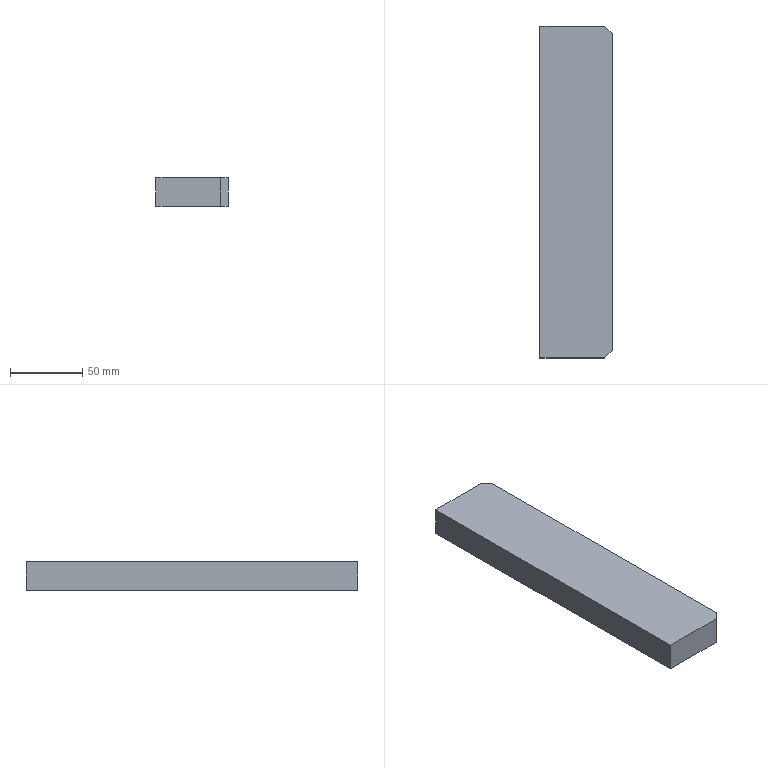Part | STEP file | Tube necking machine_id722_x_t | 1 solid | 8 faces | box 50 x 230 x 20 mm | volume 229500 mm3 | plane 8
STEP:
#1=CARTESIAN_POINT('',(0.,0.,0.));
#2=DIRECTION('',(0.,0.,1.));
#3=DIRECTION('',(1.,0.,0.));
#4=AXIS2_PLACEMENT_3D('',#1,#2,#3);
#5=CARTESIAN_POINT('',(222.5,-271.,20.));
#6=VERTEX_POINT('',#5);
#7=CARTESIAN_POINT('',(222.5,-51.,20.));
#8=VERTEX_POINT('',#7);
#9=CARTESIAN_POINT('',(222.5,-46.,20.));
#10=DIRECTION('',(0.,1.,0.));
#11=VECTOR('',#10,1.);
#12=LINE('',#9,#11);
#13=CARTESIAN_POINT('',(222.5,-46.,20.));
#14=DIRECTION('',(-1.,0.,0.));
#15=DIRECTION('',(0.,1.,0.));
#16=AXIS2_PLACEMENT_3D('',#13,#14,#15);
#17=PLANE('',#16);
#18=CARTESIAN_POINT('',(0.,0.));
#19=DIRECTION('',(1.,0.));
#20=VECTOR('',#19,1.);
#21=LINE('',#18,#20);
#22=(GEOMETRIC_REPRESENTATION_CONTEXT(2)PARAMETRIC_REPRESENTATION_CONTEXT()REPRESENTATION_CONTEXT('',''));
#23=DEFINITIONAL_REPRESENTATION('',(#21),#22);
#24=PCURVE('',#17,#23);
#25=CARTESIAN_POINT('',(0.,0.,20.));
#26=DIRECTION('',(0.,0.,1.));
#27=DIRECTION('',(-1.,0.,0.));
#28=AXIS2_PLACEMENT_3D('',#25,#26,#27);
#29=PLANE('',#28);
#30=CARTESIAN_POINT('',(-222.5,46.));
#31=DIRECTION('',(0.,-1.));
#32=VECTOR('',#31,1.);
#33=LINE('',#30,#32);
#34=(GEOMETRIC_REPRESENTATION_CONTEXT(2)PARAMETRIC_REPRESENTATION_CONTEXT()REPRESENTATION_CONTEXT('',''));
#35=DEFINITIONAL_REPRESENTATION('',(#33),#34);
#36=PCURVE('',#29,#35);
#37=SURFACE_CURVE('',#12,(#24,#36),.PCURVE_S1.);
#38=EDGE_CURVE('',#6,#8,#37,.T.);
#39=ORIENTED_EDGE('',*,*,#38,.F.);
#40=CARTESIAN_POINT('',(222.5,-271.,0.));
#41=VERTEX_POINT('',#40);
#42=CARTESIAN_POINT('',(222.5,-271.,20.));
#43=DIRECTION('',(0.,0.,-1.));
#44=VECTOR('',#43,1.);
#45=LINE('',#42,#44);
#46=CARTESIAN_POINT('',(-225.,0.));
#47=DIRECTION('',(0.,1.));
#48=VECTOR('',#47,1.);
#49=LINE('',#46,#48);
#50=(GEOMETRIC_REPRESENTATION_CONTEXT(2)PARAMETRIC_REPRESENTATION_CONTEXT()REPRESENTATION_CONTEXT('',''));
#51=DEFINITIONAL_REPRESENTATION('',(#49),#50);
#52=PCURVE('',#17,#51);
#53=CARTESIAN_POINT('',(217.5,-276.,20.));
#54=DIRECTION('',(-0.7071,0.7071,0.));
#55=DIRECTION('',(0.,0.,-1.));
#56=AXIS2_PLACEMENT_3D('',#53,#54,#55);
#57=PLANE('',#56);
#58=CARTESIAN_POINT('',(0.,-7.071));
#59=DIRECTION('',(1.,0.));
#60=VECTOR('',#59,1.);
#61=LINE('',#58,#60);
#62=(GEOMETRIC_REPRESENTATION_CONTEXT(2)PARAMETRIC_REPRESENTATION_CONTEXT()REPRESENTATION_CONTEXT('',''));
#63=DEFINITIONAL_REPRESENTATION('',(#61),#62);
#64=PCURVE('',#57,#63);
#65=SURFACE_CURVE('',#45,(#52,#64),.PCURVE_S1.);
#66=EDGE_CURVE('',#6,#41,#65,.T.);
#67=ORIENTED_EDGE('',*,*,#66,.T.);
#68=CARTESIAN_POINT('',(222.5,-51.,0.));
#69=VERTEX_POINT('',#68);
#70=CARTESIAN_POINT('',(222.5,-46.,0.));
#71=DIRECTION('',(0.,1.,0.));
#72=VECTOR('',#71,1.);
#73=LINE('',#70,#72);
#74=CARTESIAN_POINT('',(0.,20.));
#75=DIRECTION('',(1.,0.));
#76=VECTOR('',#75,1.);
#77=LINE('',#74,#76);
#78=(GEOMETRIC_REPRESENTATION_CONTEXT(2)PARAMETRIC_REPRESENTATION_CONTEXT()REPRESENTATION_CONTEXT('',''));
#79=DEFINITIONAL_REPRESENTATION('',(#77),#78);
#80=PCURVE('',#17,#79);
#81=CARTESIAN_POINT('',(0.,0.,0.));
#82=DIRECTION('',(0.,0.,1.));
#83=DIRECTION('',(-1.,0.,0.));
#84=AXIS2_PLACEMENT_3D('',#81,#82,#83);
#85=PLANE('',#84);
#86=CARTESIAN_POINT('',(-222.5,46.));
#87=DIRECTION('',(0.,-1.));
#88=VECTOR('',#87,1.);
#89=LINE('',#86,#88);
#90=(GEOMETRIC_REPRESENTATION_CONTEXT(2)PARAMETRIC_REPRESENTATION_CONTEXT()REPRESENTATION_CONTEXT('',''));
#91=DEFINITIONAL_REPRESENTATION('',(#89),#90);
#92=PCURVE('',#85,#91);
#93=SURFACE_CURVE('',#73,(#80,#92),.PCURVE_S1.);
#94=EDGE_CURVE('',#41,#69,#93,.T.);
#95=ORIENTED_EDGE('',*,*,#94,.T.);
#96=CARTESIAN_POINT('',(222.5,-51.,20.));
#97=DIRECTION('',(0.,0.,1.));
#98=VECTOR('',#97,1.);
#99=LINE('',#96,#98);
#100=CARTESIAN_POINT('',(-5.,0.));
#101=DIRECTION('',(0.,-1.));
#102=VECTOR('',#101,1.);
#103=LINE('',#100,#102);
#104=(GEOMETRIC_REPRESENTATION_CONTEXT(2)PARAMETRIC_REPRESENTATION_CONTEXT()REPRESENTATION_CONTEXT('',''));
#105=DEFINITIONAL_REPRESENTATION('',(#103),#104);
#106=PCURVE('',#17,#105);
#107=CARTESIAN_POINT('',(222.5,-51.,20.));
#108=DIRECTION('',(-0.7071,-0.7071,0.));
#109=DIRECTION('',(0.,0.,-1.));
#110=AXIS2_PLACEMENT_3D('',#107,#108,#109);
#111=PLANE('',#110);
#112=CARTESIAN_POINT('',(0.,0.));
#113=DIRECTION('',(-1.,0.));
#114=VECTOR('',#113,1.);
#115=LINE('',#112,#114);
#116=(GEOMETRIC_REPRESENTATION_CONTEXT(2)PARAMETRIC_REPRESENTATION_CONTEXT()REPRESENTATION_CONTEXT('',''));
#117=DEFINITIONAL_REPRESENTATION('',(#115),#116);
#118=PCURVE('',#111,#117);
#119=SURFACE_CURVE('',#99,(#106,#118),.PCURVE_S1.);
#120=EDGE_CURVE('',#69,#8,#119,.T.);
#121=ORIENTED_EDGE('',*,*,#120,.T.);
#122=EDGE_LOOP('',(#39,#67,#95,#121));
#123=FACE_BOUND('',#122,.T.);
#124=ADVANCED_FACE('',(#123),#17,.F.);
#125=CARTESIAN_POINT('',(172.5,-276.,20.));
#126=VERTEX_POINT('',#125);
#127=CARTESIAN_POINT('',(217.5,-276.,20.));
#128=VERTEX_POINT('',#127);
#129=CARTESIAN_POINT('',(222.5,-276.,20.));
#130=DIRECTION('',(1.,0.,0.));
#131=VECTOR('',#130,1.);
#132=LINE('',#129,#131);
#133=CARTESIAN_POINT('',(222.5,-276.,20.));
#134=DIRECTION('',(0.,1.,0.));
#135=DIRECTION('',(1.,0.,0.));
#136=AXIS2_PLACEMENT_3D('',#133,#134,#135);
#137=PLANE('',#136);
#138=CARTESIAN_POINT('',(0.,0.));
#139=DIRECTION('',(1.,0.));
#140=VECTOR('',#139,1.);
#141=LINE('',#138,#140);
#142=(GEOMETRIC_REPRESENTATION_CONTEXT(2)PARAMETRIC_REPRESENTATION_CONTEXT()REPRESENTATION_CONTEXT('',''));
#143=DEFINITIONAL_REPRESENTATION('',(#141),#142);
#144=PCURVE('',#137,#143);
#145=CARTESIAN_POINT('',(-222.5,276.));
#146=DIRECTION('',(-1.,0.));
#147=VECTOR('',#146,1.);
#148=LINE('',#145,#147);
#149=(GEOMETRIC_REPRESENTATION_CONTEXT(2)PARAMETRIC_REPRESENTATION_CONTEXT()REPRESENTATION_CONTEXT('',''));
#150=DEFINITIONAL_REPRESENTATION('',(#148),#149);
#151=PCURVE('',#29,#150);
#152=SURFACE_CURVE('',#132,(#144,#151),.PCURVE_S1.);
#153=EDGE_CURVE('',#126,#128,#152,.T.);
#154=ORIENTED_EDGE('',*,*,#153,.F.);
#155=CARTESIAN_POINT('',(172.5,-276.,0.));
#156=VERTEX_POINT('',#155);
#157=CARTESIAN_POINT('',(172.5,-276.,20.));
#158=DIRECTION('',(0.,0.,1.));
#159=VECTOR('',#158,1.);
#160=LINE('',#157,#159);
#161=CARTESIAN_POINT('',(-50.,0.));
#162=DIRECTION('',(0.,-1.));
#163=VECTOR('',#162,1.);
#164=LINE('',#161,#163);
#165=(GEOMETRIC_REPRESENTATION_CONTEXT(2)PARAMETRIC_REPRESENTATION_CONTEXT()REPRESENTATION_CONTEXT('',''));
#166=DEFINITIONAL_REPRESENTATION('',(#164),#165);
#167=PCURVE('',#137,#166);
#168=CARTESIAN_POINT('',(172.5,-276.,20.));
#169=DIRECTION('',(1.,0.,0.));
#170=DIRECTION('',(0.,-1.,0.));
#171=AXIS2_PLACEMENT_3D('',#168,#169,#170);
#172=PLANE('',#171);
#173=CARTESIAN_POINT('',(0.,0.));
#174=DIRECTION('',(0.,-1.));
#175=VECTOR('',#174,1.);
#176=LINE('',#173,#175);
#177=(GEOMETRIC_REPRESENTATION_CONTEXT(2)PARAMETRIC_REPRESENTATION_CONTEXT()REPRESENTATION_CONTEXT('',''));
#178=DEFINITIONAL_REPRESENTATION('',(#176),#177);
#179=PCURVE('',#172,#178);
#180=SURFACE_CURVE('',#160,(#167,#179),.PCURVE_S1.);
#181=EDGE_CURVE('',#156,#126,#180,.T.);
#182=ORIENTED_EDGE('',*,*,#181,.F.);
#183=CARTESIAN_POINT('',(217.5,-276.,0.));
#184=VERTEX_POINT('',#183);
#185=CARTESIAN_POINT('',(222.5,-276.,0.));
#186=DIRECTION('',(1.,0.,0.));
#187=VECTOR('',#186,1.);
#188=LINE('',#185,#187);
#189=CARTESIAN_POINT('',(0.,20.));
#190=DIRECTION('',(1.,0.));
#191=VECTOR('',#190,1.);
#192=LINE('',#189,#191);
#193=(GEOMETRIC_REPRESENTATION_CONTEXT(2)PARAMETRIC_REPRESENTATION_CONTEXT()REPRESENTATION_CONTEXT('',''));
#194=DEFINITIONAL_REPRESENTATION('',(#192),#193);
#195=PCURVE('',#137,#194);
#196=CARTESIAN_POINT('',(-222.5,276.));
#197=DIRECTION('',(-1.,0.));
#198=VECTOR('',#197,1.);
#199=LINE('',#196,#198);
#200=(GEOMETRIC_REPRESENTATION_CONTEXT(2)PARAMETRIC_REPRESENTATION_CONTEXT()REPRESENTATION_CONTEXT('',''));
#201=DEFINITIONAL_REPRESENTATION('',(#199),#200);
#202=PCURVE('',#85,#201);
#203=SURFACE_CURVE('',#188,(#195,#202),.PCURVE_S1.);
#204=EDGE_CURVE('',#156,#184,#203,.T.);
#205=ORIENTED_EDGE('',*,*,#204,.T.);
#206=CARTESIAN_POINT('',(217.5,-276.,20.));
#207=DIRECTION('',(0.,0.,1.));
#208=VECTOR('',#207,1.);
#209=LINE('',#206,#208);
#210=CARTESIAN_POINT('',(-5.,0.));
#211=DIRECTION('',(0.,-1.));
#212=VECTOR('',#211,1.);
#213=LINE('',#210,#212);
#214=(GEOMETRIC_REPRESENTATION_CONTEXT(2)PARAMETRIC_REPRESENTATION_CONTEXT()REPRESENTATION_CONTEXT('',''));
#215=DEFINITIONAL_REPRESENTATION('',(#213),#214);
#216=PCURVE('',#137,#215);
#217=CARTESIAN_POINT('',(0.,0.));
#218=DIRECTION('',(-1.,0.));
#219=VECTOR('',#218,1.);
#220=LINE('',#217,#219);
#221=(GEOMETRIC_REPRESENTATION_CONTEXT(2)PARAMETRIC_REPRESENTATION_CONTEXT()REPRESENTATION_CONTEXT('',''));
#222=DEFINITIONAL_REPRESENTATION('',(#220),#221);
#223=PCURVE('',#57,#222);
#224=SURFACE_CURVE('',#209,(#216,#223),.PCURVE_S1.);
#225=EDGE_CURVE('',#184,#128,#224,.T.);
#226=ORIENTED_EDGE('',*,*,#225,.T.);
#227=EDGE_LOOP('',(#154,#182,#205,#226));
#228=FACE_BOUND('',#227,.T.);
#229=ADVANCED_FACE('',(#228),#137,.F.);
#230=CARTESIAN_POINT('',(172.5,-46.,0.));
#231=VERTEX_POINT('',#230);
#232=CARTESIAN_POINT('',(172.5,-276.,0.));
#233=DIRECTION('',(0.,-1.,0.));
#234=VECTOR('',#233,1.);
#235=LINE('',#232,#234);
#236=CARTESIAN_POINT('',(0.,20.));
#237=DIRECTION('',(1.,0.));
#238=VECTOR('',#237,1.);
#239=LINE('',#236,#238);
#240=(GEOMETRIC_REPRESENTATION_CONTEXT(2)PARAMETRIC_REPRESENTATION_CONTEXT()REPRESENTATION_CONTEXT('',''));
#241=DEFINITIONAL_REPRESENTATION('',(#239),#240);
#242=PCURVE('',#172,#241);
#243=CARTESIAN_POINT('',(-172.5,276.));
#244=DIRECTION('',(0.,1.));
#245=VECTOR('',#244,1.);
#246=LINE('',#243,#245);
#247=(GEOMETRIC_REPRESENTATION_CONTEXT(2)PARAMETRIC_REPRESENTATION_CONTEXT()REPRESENTATION_CONTEXT('',''));
#248=DEFINITIONAL_REPRESENTATION('',(#246),#247);
#249=PCURVE('',#85,#248);
#250=SURFACE_CURVE('',#235,(#242,#249),.PCURVE_S1.);
#251=EDGE_CURVE('',#231,#156,#250,.T.);
#252=ORIENTED_EDGE('',*,*,#251,.T.);
#253=ORIENTED_EDGE('',*,*,#181,.T.);
#254=CARTESIAN_POINT('',(172.5,-46.,20.));
#255=VERTEX_POINT('',#254);
#256=CARTESIAN_POINT('',(172.5,-276.,20.));
#257=DIRECTION('',(0.,-1.,0.));
#258=VECTOR('',#257,1.);
#259=LINE('',#256,#258);
#260=CARTESIAN_POINT('',(0.,0.));
#261=DIRECTION('',(1.,0.));
#262=VECTOR('',#261,1.);
#263=LINE('',#260,#262);
#264=(GEOMETRIC_REPRESENTATION_CONTEXT(2)PARAMETRIC_REPRESENTATION_CONTEXT()REPRESENTATION_CONTEXT('',''));
#265=DEFINITIONAL_REPRESENTATION('',(#263),#264);
#266=PCURVE('',#172,#265);
#267=CARTESIAN_POINT('',(-172.5,276.));
#268=DIRECTION('',(0.,1.));
#269=VECTOR('',#268,1.);
#270=LINE('',#267,#269);
#271=(GEOMETRIC_REPRESENTATION_CONTEXT(2)PARAMETRIC_REPRESENTATION_CONTEXT()REPRESENTATION_CONTEXT('',''));
#272=DEFINITIONAL_REPRESENTATION('',(#270),#271);
#273=PCURVE('',#29,#272);
#274=SURFACE_CURVE('',#259,(#266,#273),.PCURVE_S1.);
#275=EDGE_CURVE('',#255,#126,#274,.T.);
#276=ORIENTED_EDGE('',*,*,#275,.F.);
#277=CARTESIAN_POINT('',(172.5,-46.,20.));
#278=DIRECTION('',(0.,0.,1.));
#279=VECTOR('',#278,1.);
#280=LINE('',#277,#279);
#281=CARTESIAN_POINT('',(-230.,0.));
#282=DIRECTION('',(0.,-1.));
#283=VECTOR('',#282,1.);
#284=LINE('',#281,#283);
#285=(GEOMETRIC_REPRESENTATION_CONTEXT(2)PARAMETRIC_REPRESENTATION_CONTEXT()REPRESENTATION_CONTEXT('',''));
#286=DEFINITIONAL_REPRESENTATION('',(#284),#285);
#287=PCURVE('',#172,#286);
#288=CARTESIAN_POINT('',(172.5,-46.,20.));
#289=DIRECTION('',(0.,-1.,0.));
#290=DIRECTION('',(-1.,0.,0.));
#291=AXIS2_PLACEMENT_3D('',#288,#289,#290);
#292=PLANE('',#291);
#293=CARTESIAN_POINT('',(0.,0.));
#294=DIRECTION('',(0.,-1.));
#295=VECTOR('',#294,1.);
#296=LINE('',#293,#295);
#297=(GEOMETRIC_REPRESENTATION_CONTEXT(2)PARAMETRIC_REPRESENTATION_CONTEXT()REPRESENTATION_CONTEXT('',''));
#298=DEFINITIONAL_REPRESENTATION('',(#296),#297);
#299=PCURVE('',#292,#298);
#300=SURFACE_CURVE('',#280,(#287,#299),.PCURVE_S1.);
#301=EDGE_CURVE('',#231,#255,#300,.T.);
#302=ORIENTED_EDGE('',*,*,#301,.F.);
#303=EDGE_LOOP('',(#252,#253,#276,#302));
#304=FACE_BOUND('',#303,.T.);
#305=ADVANCED_FACE('',(#304),#172,.F.);
#306=CARTESIAN_POINT('',(217.5,-46.,0.));
#307=VERTEX_POINT('',#306);
#308=CARTESIAN_POINT('',(172.5,-46.,0.));
#309=DIRECTION('',(-1.,0.,0.));
#310=VECTOR('',#309,1.);
#311=LINE('',#308,#310);
#312=CARTESIAN_POINT('',(0.,20.));
#313=DIRECTION('',(1.,0.));
#314=VECTOR('',#313,1.);
#315=LINE('',#312,#314);
#316=(GEOMETRIC_REPRESENTATION_CONTEXT(2)PARAMETRIC_REPRESENTATION_CONTEXT()REPRESENTATION_CONTEXT('',''));
#317=DEFINITIONAL_REPRESENTATION('',(#315),#316);
#318=PCURVE('',#292,#317);
#319=CARTESIAN_POINT('',(-172.5,46.));
#320=DIRECTION('',(1.,0.));
#321=VECTOR('',#320,1.);
#322=LINE('',#319,#321);
#323=(GEOMETRIC_REPRESENTATION_CONTEXT(2)PARAMETRIC_REPRESENTATION_CONTEXT()REPRESENTATION_CONTEXT('',''));
#324=DEFINITIONAL_REPRESENTATION('',(#322),#323);
#325=PCURVE('',#85,#324);
#326=SURFACE_CURVE('',#311,(#318,#325),.PCURVE_S1.);
#327=EDGE_CURVE('',#307,#231,#326,.T.);
#328=ORIENTED_EDGE('',*,*,#327,.T.);
#329=ORIENTED_EDGE('',*,*,#301,.T.);
#330=CARTESIAN_POINT('',(217.5,-46.,20.));
#331=VERTEX_POINT('',#330);
#332=CARTESIAN_POINT('',(172.5,-46.,20.));
#333=DIRECTION('',(-1.,0.,0.));
#334=VECTOR('',#333,1.);
#335=LINE('',#332,#334);
#336=CARTESIAN_POINT('',(0.,0.));
#337=DIRECTION('',(1.,0.));
#338=VECTOR('',#337,1.);
#339=LINE('',#336,#338);
#340=(GEOMETRIC_REPRESENTATION_CONTEXT(2)PARAMETRIC_REPRESENTATION_CONTEXT()REPRESENTATION_CONTEXT('',''));
#341=DEFINITIONAL_REPRESENTATION('',(#339),#340);
#342=PCURVE('',#292,#341);
#343=CARTESIAN_POINT('',(-172.5,46.));
#344=DIRECTION('',(1.,0.));
#345=VECTOR('',#344,1.);
#346=LINE('',#343,#345);
#347=(GEOMETRIC_REPRESENTATION_CONTEXT(2)PARAMETRIC_REPRESENTATION_CONTEXT()REPRESENTATION_CONTEXT('',''));
#348=DEFINITIONAL_REPRESENTATION('',(#346),#347);
#349=PCURVE('',#29,#348);
#350=SURFACE_CURVE('',#335,(#342,#349),.PCURVE_S1.);
#351=EDGE_CURVE('',#331,#255,#350,.T.);
#352=ORIENTED_EDGE('',*,*,#351,.F.);
#353=CARTESIAN_POINT('',(217.5,-46.,20.));
#354=DIRECTION('',(0.,0.,-1.));
#355=VECTOR('',#354,1.);
#356=LINE('',#353,#355);
#357=CARTESIAN_POINT('',(-45.,0.));
#358=DIRECTION('',(0.,1.));
#359=VECTOR('',#358,1.);
#360=LINE('',#357,#359);
#361=(GEOMETRIC_REPRESENTATION_CONTEXT(2)PARAMETRIC_REPRESENTATION_CONTEXT()REPRESENTATION_CONTEXT('',''));
#362=DEFINITIONAL_REPRESENTATION('',(#360),#361);
#363=PCURVE('',#292,#362);
#364=CARTESIAN_POINT('',(0.,-7.071));
#365=DIRECTION('',(1.,0.));
#366=VECTOR('',#365,1.);
#367=LINE('',#364,#366);
#368=(GEOMETRIC_REPRESENTATION_CONTEXT(2)PARAMETRIC_REPRESENTATION_CONTEXT()REPRESENTATION_CONTEXT('',''));
#369=DEFINITIONAL_REPRESENTATION('',(#367),#368);
#370=PCURVE('',#111,#369);
#371=SURFACE_CURVE('',#356,(#363,#370),.PCURVE_S1.);
#372=EDGE_CURVE('',#331,#307,#371,.T.);
#373=ORIENTED_EDGE('',*,*,#372,.T.);
#374=EDGE_LOOP('',(#328,#329,#352,#373));
#375=FACE_BOUND('',#374,.T.);
#376=ADVANCED_FACE('',(#375),#292,.F.);
#377=ORIENTED_EDGE('',*,*,#351,.T.);
#378=ORIENTED_EDGE('',*,*,#275,.T.);
#379=ORIENTED_EDGE('',*,*,#153,.T.);
#380=CARTESIAN_POINT('',(246.75,-246.75,20.));
#381=DIRECTION('',(0.7071,0.7071,0.));
#382=VECTOR('',#381,1.);
#383=LINE('',#380,#382);
#384=CARTESIAN_POINT('',(-246.75,246.75));
#385=DIRECTION('',(-0.7071,-0.7071));
#386=VECTOR('',#385,1.);
#387=LINE('',#384,#386);
#388=(GEOMETRIC_REPRESENTATION_CONTEXT(2)PARAMETRIC_REPRESENTATION_CONTEXT()REPRESENTATION_CONTEXT('',''));
#389=DEFINITIONAL_REPRESENTATION('',(#387),#388);
#390=PCURVE('',#29,#389);
#391=CARTESIAN_POINT('',(0.,-41.366));
#392=DIRECTION('',(0.,-1.));
#393=VECTOR('',#392,1.);
#394=LINE('',#391,#393);
#395=(GEOMETRIC_REPRESENTATION_CONTEXT(2)PARAMETRIC_REPRESENTATION_CONTEXT()REPRESENTATION_CONTEXT('',''));
#396=DEFINITIONAL_REPRESENTATION('',(#394),#395);
#397=PCURVE('',#57,#396);
#398=SURFACE_CURVE('',#383,(#390,#397),.PCURVE_S1.);
#399=EDGE_CURVE('',#128,#6,#398,.T.);
#400=ORIENTED_EDGE('',*,*,#399,.T.);
#401=ORIENTED_EDGE('',*,*,#38,.T.);
#402=CARTESIAN_POINT('',(85.75,85.75,20.));
#403=DIRECTION('',(-0.7071,0.7071,0.));
#404=VECTOR('',#403,1.);
#405=LINE('',#402,#404);
#406=CARTESIAN_POINT('',(-85.75,-85.75));
#407=DIRECTION('',(0.7071,-0.7071));
#408=VECTOR('',#407,1.);
#409=LINE('',#406,#408);
#410=(GEOMETRIC_REPRESENTATION_CONTEXT(2)PARAMETRIC_REPRESENTATION_CONTEXT()REPRESENTATION_CONTEXT('',''));
#411=DEFINITIONAL_REPRESENTATION('',(#409),#410);
#412=PCURVE('',#29,#411);
#413=CARTESIAN_POINT('',(0.,-193.394));
#414=DIRECTION('',(0.,-1.));
#415=VECTOR('',#414,1.);
#416=LINE('',#413,#415);
#417=(GEOMETRIC_REPRESENTATION_CONTEXT(2)PARAMETRIC_REPRESENTATION_CONTEXT()REPRESENTATION_CONTEXT('',''));
#418=DEFINITIONAL_REPRESENTATION('',(#416),#417);
#419=PCURVE('',#111,#418);
#420=SURFACE_CURVE('',#405,(#412,#419),.PCURVE_S1.);
#421=EDGE_CURVE('',#8,#331,#420,.T.);
#422=ORIENTED_EDGE('',*,*,#421,.T.);
#423=EDGE_LOOP('',(#377,#378,#379,#400,#401,#422));
#424=FACE_BOUND('',#423,.T.);
#425=ADVANCED_FACE('',(#424),#29,.T.);
#426=ORIENTED_EDGE('',*,*,#94,.F.);
#427=CARTESIAN_POINT('',(217.5,-276.,0.));
#428=DIRECTION('',(-0.7071,-0.7071,0.));
#429=VECTOR('',#428,1.);
#430=LINE('',#427,#429);
#431=CARTESIAN_POINT('',(-217.5,276.));
#432=DIRECTION('',(0.7071,0.7071));
#433=VECTOR('',#432,1.);
#434=LINE('',#431,#433);
#435=(GEOMETRIC_REPRESENTATION_CONTEXT(2)PARAMETRIC_REPRESENTATION_CONTEXT()REPRESENTATION_CONTEXT('',''));
#436=DEFINITIONAL_REPRESENTATION('',(#434),#435);
#437=PCURVE('',#85,#436);
#438=CARTESIAN_POINT('',(20.,0.));
#439=DIRECTION('',(0.,1.));
#440=VECTOR('',#439,1.);
#441=LINE('',#438,#440);
#442=(GEOMETRIC_REPRESENTATION_CONTEXT(2)PARAMETRIC_REPRESENTATION_CONTEXT()REPRESENTATION_CONTEXT('',''));
#443=DEFINITIONAL_REPRESENTATION('',(#441),#442);
#444=PCURVE('',#57,#443);
#445=SURFACE_CURVE('',#430,(#437,#444),.PCURVE_S1.);
#446=EDGE_CURVE('',#41,#184,#445,.T.);
#447=ORIENTED_EDGE('',*,*,#446,.T.);
#448=ORIENTED_EDGE('',*,*,#204,.F.);
#449=ORIENTED_EDGE('',*,*,#251,.F.);
#450=ORIENTED_EDGE('',*,*,#327,.F.);
#451=CARTESIAN_POINT('',(222.5,-51.,0.));
#452=DIRECTION('',(0.7071,-0.7071,0.));
#453=VECTOR('',#452,1.);
#454=LINE('',#451,#453);
#455=CARTESIAN_POINT('',(-222.5,51.));
#456=DIRECTION('',(-0.7071,0.7071));
#457=VECTOR('',#456,1.);
#458=LINE('',#455,#457);
#459=(GEOMETRIC_REPRESENTATION_CONTEXT(2)PARAMETRIC_REPRESENTATION_CONTEXT()REPRESENTATION_CONTEXT('',''));
#460=DEFINITIONAL_REPRESENTATION('',(#458),#459);
#461=PCURVE('',#85,#460);
#462=CARTESIAN_POINT('',(20.,0.));
#463=DIRECTION('',(0.,1.));
#464=VECTOR('',#463,1.);
#465=LINE('',#462,#464);
#466=(GEOMETRIC_REPRESENTATION_CONTEXT(2)PARAMETRIC_REPRESENTATION_CONTEXT()REPRESENTATION_CONTEXT('',''));
#467=DEFINITIONAL_REPRESENTATION('',(#465),#466);
#468=PCURVE('',#111,#467);
#469=SURFACE_CURVE('',#454,(#461,#468),.PCURVE_S1.);
#470=EDGE_CURVE('',#307,#69,#469,.T.);
#471=ORIENTED_EDGE('',*,*,#470,.T.);
#472=EDGE_LOOP('',(#426,#447,#448,#449,#450,#471));
#473=FACE_BOUND('',#472,.T.);
#474=ADVANCED_FACE('',(#473),#85,.F.);
#475=ORIENTED_EDGE('',*,*,#421,.F.);
#476=ORIENTED_EDGE('',*,*,#120,.F.);
#477=ORIENTED_EDGE('',*,*,#470,.F.);
#478=ORIENTED_EDGE('',*,*,#372,.F.);
#479=EDGE_LOOP('',(#475,#476,#477,#478));
#480=FACE_BOUND('',#479,.T.);
#481=ADVANCED_FACE('',(#480),#111,.F.);
#482=ORIENTED_EDGE('',*,*,#399,.F.);
#483=ORIENTED_EDGE('',*,*,#225,.F.);
#484=ORIENTED_EDGE('',*,*,#446,.F.);
#485=ORIENTED_EDGE('',*,*,#66,.F.);
#486=EDGE_LOOP('',(#482,#483,#484,#485));
#487=FACE_BOUND('',#486,.T.);
#488=ADVANCED_FACE('',(#487),#57,.F.);
#489=CLOSED_SHELL('',(#124,#229,#305,#376,#425,#474,#481,#488));
#490=MANIFOLD_SOLID_BREP('',#489);
#491=(LENGTH_UNIT()NAMED_UNIT(*)SI_UNIT(.MILLI.,.METRE.));
#492=UNCERTAINTY_MEASURE_WITH_UNIT(LENGTH_MEASURE(0.0000001),#491,'','');
#493=(NAMED_UNIT(*)PLANE_ANGLE_UNIT()SI_UNIT($,.RADIAN.));
#494=(NAMED_UNIT(*)SI_UNIT($,.STERADIAN.)SOLID_ANGLE_UNIT());
#495=(GEOMETRIC_REPRESENTATION_CONTEXT(3)GLOBAL_UNCERTAINTY_ASSIGNED_CONTEXT((#492))GLOBAL_UNIT_ASSIGNED_CONTEXT((#491,#493,#494))REPRESENTATION_CONTEXT('',''));
#496=ADVANCED_BREP_SHAPE_REPRESENTATION('',(#4,#490),#495);